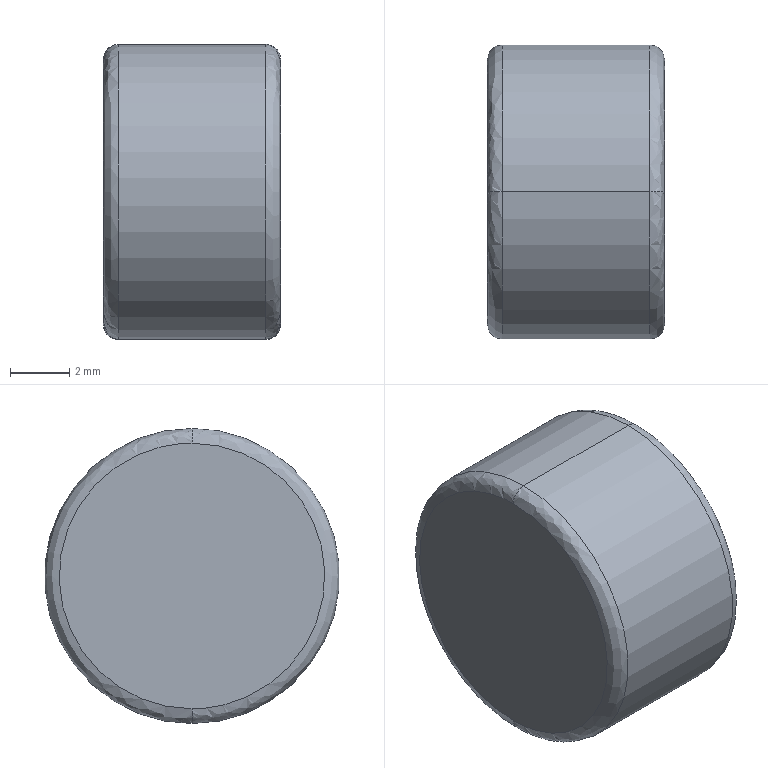Part | STEP file | Magnet dia 10 thickness 6 | 1 solid | 8 faces | box 6 x 10 x 10 mm | volume 467.969 mm3 | spline 4 | cylinder 2 | plane 2 | commonest cylinder face diameters 10 x2
STEP:
#1=CARTESIAN_POINT('',(0.,0.,0.));
#2=DIRECTION('',(0.,0.,1.));
#3=DIRECTION('',(1.,0.,0.));
#4=AXIS2_PLACEMENT_3D('',#1,#2,#3);
#5=CARTESIAN_POINT('',(5.5,-0.000000001,-5.));
#6=VERTEX_POINT('',#5);
#7=CARTESIAN_POINT('',(5.5,0.,5.));
#8=VERTEX_POINT('',#7);
#9=CARTESIAN_POINT('',(5.5,0.,0.));
#10=DIRECTION('',(1.,0.,0.));
#11=DIRECTION('',(0.,0.,1.));
#12=AXIS2_PLACEMENT_3D('',#9,#10,#11);
#13=CIRCLE('',#12,5.);
#14=CARTESIAN_POINT('',(5.5,0.,0.));
#15=DIRECTION('',(-1.,0.,0.));
#16=DIRECTION('',(0.,0.,1.));
#17=AXIS2_PLACEMENT_3D('',#14,#15,#16);
#18=CYLINDRICAL_SURFACE('',#17,5.);
#19=CARTESIAN_POINT('',(6.283,0.));
#20=DIRECTION('',(-1.,0.));
#21=VECTOR('',#20,1.);
#22=LINE('',#19,#21);
#23=(GEOMETRIC_REPRESENTATION_CONTEXT(2)PARAMETRIC_REPRESENTATION_CONTEXT()REPRESENTATION_CONTEXT('',''));
#24=DEFINITIONAL_REPRESENTATION('',(#22),#23);
#25=PCURVE('',#18,#24);
#26=CARTESIAN_POINT('',(5.998,0.,-4.45));
#27=CARTESIAN_POINT('',(5.998,8.9,-4.45));
#28=CARTESIAN_POINT('',(5.998,8.9,4.45));
#29=CARTESIAN_POINT('',(5.998,0.,4.45));
#30=CARTESIAN_POINT('',(6.032,0.,-4.79));
#31=CARTESIAN_POINT('',(6.032,9.58,-4.79));
#32=CARTESIAN_POINT('',(6.032,9.58,4.79));
#33=CARTESIAN_POINT('',(6.032,0.,4.79));
#34=CARTESIAN_POINT('',(5.79,0.,-5.032));
#35=CARTESIAN_POINT('',(5.79,10.063,-5.032));
#36=CARTESIAN_POINT('',(5.79,10.063,5.032));
#37=CARTESIAN_POINT('',(5.79,0.,5.032));
#38=CARTESIAN_POINT('',(5.45,0.,-4.998));
#39=CARTESIAN_POINT('',(5.45,9.995,-4.998));
#40=CARTESIAN_POINT('',(5.45,9.995,4.998));
#41=CARTESIAN_POINT('',(5.45,0.,4.998));
#42=(BOUNDED_SURFACE()B_SPLINE_SURFACE(3,3,((#26,#27,#28,#29),(#30,#31,#32,#33),(#34,#35,#36,#37),(#38,#39,#40,#41)),.UNSPECIFIED.,.F.,.F.,.F.)B_SPLINE_SURFACE_WITH_KNOTS((4,4),(4,4),(0.,1.),(0.,1.),.PIECEWISE_BEZIER_KNOTS.)GEOMETRIC_REPRESENTATION_ITEM()RATIONAL_B_SPLINE_SURFACE(((1.,0.3333,0.3333,1.),(0.7553,0.2518,0.2518,0.7553),(0.7553,0.2518,0.2518,0.7553),(1.,0.3333,0.3333,1.)))REPRESENTATION_ITEM('')SURFACE());
#43=CARTESIAN_POINT('',(0.9369,0.));
#44=CARTESIAN_POINT('',(0.9369,0.02375));
#45=CARTESIAN_POINT('',(0.9369,0.06805));
#46=CARTESIAN_POINT('',(0.9369,0.1267));
#47=CARTESIAN_POINT('',(0.9369,0.1794));
#48=CARTESIAN_POINT('',(0.9369,0.2276));
#49=CARTESIAN_POINT('',(0.9369,0.2721));
#50=CARTESIAN_POINT('',(0.9369,0.3139));
#51=CARTESIAN_POINT('',(0.9369,0.3535));
#52=CARTESIAN_POINT('',(0.9369,0.3914));
#53=CARTESIAN_POINT('',(0.9369,0.4282));
#54=CARTESIAN_POINT('',(0.9369,0.4643));
#55=CARTESIAN_POINT('',(0.9369,0.5));
#56=CARTESIAN_POINT('',(0.9369,0.5357));
#57=CARTESIAN_POINT('',(0.9369,0.5718));
#58=CARTESIAN_POINT('',(0.9369,0.6086));
#59=CARTESIAN_POINT('',(0.9369,0.6465));
#60=CARTESIAN_POINT('',(0.9369,0.6861));
#61=CARTESIAN_POINT('',(0.9369,0.7279));
#62=CARTESIAN_POINT('',(0.9369,0.7724));
#63=CARTESIAN_POINT('',(0.9369,0.8206));
#64=CARTESIAN_POINT('',(0.9369,0.8733));
#65=CARTESIAN_POINT('',(0.9369,0.9319));
#66=CARTESIAN_POINT('',(0.9369,0.9763));
#67=CARTESIAN_POINT('',(0.9369,1.));
#68=B_SPLINE_CURVE_WITH_KNOTS('',3,(#43,#44,#45,#46,#47,#48,#49,#50,#51,#52,#53,#54,#55,#56,#57,#58,#59,#60,#61,#62,#63,#64,#65,#66,#67),.UNSPECIFIED.,.F.,.F.,(4,1,1,1,1,1,1,1,1,1,1,1,1,1,1,1,1,1,1,1,1,1,4),(3.142,3.284,3.427,3.57,3.713,3.856,3.998,4.141,4.284,4.427,4.57,4.712,4.855,4.998,5.141,5.284,5.426,5.569,5.712,5.855,5.998,6.14,6.283),.QUASI_UNIFORM_KNOTS.);
#69=(GEOMETRIC_REPRESENTATION_CONTEXT(2)PARAMETRIC_REPRESENTATION_CONTEXT()REPRESENTATION_CONTEXT('',''));
#70=DEFINITIONAL_REPRESENTATION('',(#68),#69);
#71=PCURVE('',#42,#70);
#72=SURFACE_CURVE('',#13,(#25,#71),.PCURVE_S1.);
#73=EDGE_CURVE('',#6,#8,#72,.T.);
#74=ORIENTED_EDGE('',*,*,#73,.F.);
#75=CARTESIAN_POINT('',(0.5,0.,-5.));
#76=VERTEX_POINT('',#75);
#77=CARTESIAN_POINT('',(5.5,0.,-5.));
#78=DIRECTION('',(-1.,0.,0.));
#79=VECTOR('',#78,1.);
#80=LINE('',#77,#79);
#81=CARTESIAN_POINT('',(3.142,0.));
#82=DIRECTION('',(0.,1.));
#83=VECTOR('',#82,1.);
#84=LINE('',#81,#83);
#85=(GEOMETRIC_REPRESENTATION_CONTEXT(2)PARAMETRIC_REPRESENTATION_CONTEXT()REPRESENTATION_CONTEXT('',''));
#86=DEFINITIONAL_REPRESENTATION('',(#84),#85);
#87=PCURVE('',#18,#86);
#88=CARTESIAN_POINT('',(5.5,0.,0.));
#89=DIRECTION('',(-1.,0.,0.));
#90=DIRECTION('',(0.,0.,1.));
#91=AXIS2_PLACEMENT_3D('',#88,#89,#90);
#92=CYLINDRICAL_SURFACE('',#91,5.);
#93=CARTESIAN_POINT('',(3.142,0.));
#94=DIRECTION('',(0.,1.));
#95=VECTOR('',#94,1.);
#96=LINE('',#93,#95);
#97=(GEOMETRIC_REPRESENTATION_CONTEXT(2)PARAMETRIC_REPRESENTATION_CONTEXT()REPRESENTATION_CONTEXT('',''));
#98=DEFINITIONAL_REPRESENTATION('',(#96),#97);
#99=PCURVE('',#92,#98);
#100=SURFACE_CURVE('',#80,(#87,#99),.PCURVE_S1.);
#101=EDGE_CURVE('',#6,#76,#100,.T.);
#102=ORIENTED_EDGE('',*,*,#101,.T.);
#103=CARTESIAN_POINT('',(0.5,0.,5.));
#104=VERTEX_POINT('',#103);
#105=CARTESIAN_POINT('',(0.5,0.,0.));
#106=DIRECTION('',(-1.,0.,0.));
#107=DIRECTION('',(0.,-1.,0.));
#108=AXIS2_PLACEMENT_3D('',#105,#106,#107);
#109=CIRCLE('',#108,5.);
#110=CARTESIAN_POINT('',(-1.571,5.));
#111=DIRECTION('',(1.,0.));
#112=VECTOR('',#111,1.);
#113=LINE('',#110,#112);
#114=(GEOMETRIC_REPRESENTATION_CONTEXT(2)PARAMETRIC_REPRESENTATION_CONTEXT()REPRESENTATION_CONTEXT('',''));
#115=DEFINITIONAL_REPRESENTATION('',(#113),#114);
#116=PCURVE('',#18,#115);
#117=CARTESIAN_POINT('',(0.5499,0.,-4.998));
#118=CARTESIAN_POINT('',(0.5499,9.995,-4.998));
#119=CARTESIAN_POINT('',(0.5499,9.995,4.998));
#120=CARTESIAN_POINT('',(0.5499,0.,4.998));
#121=CARTESIAN_POINT('',(0.21,0.,-5.032));
#122=CARTESIAN_POINT('',(0.21,10.063,-5.032));
#123=CARTESIAN_POINT('',(0.21,10.063,5.032));
#124=CARTESIAN_POINT('',(0.21,0.,5.032));
#125=CARTESIAN_POINT('',(-0.03161,0.,-4.79));
#126=CARTESIAN_POINT('',(-0.03161,9.58,-4.79));
#127=CARTESIAN_POINT('',(-0.03161,9.58,4.79));
#128=CARTESIAN_POINT('',(-0.03161,0.,4.79));
#129=CARTESIAN_POINT('',(0.002498,0.,-4.45));
#130=CARTESIAN_POINT('',(0.002498,8.9,-4.45));
#131=CARTESIAN_POINT('',(0.002498,8.9,4.45));
#132=CARTESIAN_POINT('',(0.002498,0.,4.45));
#133=(BOUNDED_SURFACE()B_SPLINE_SURFACE(3,3,((#117,#118,#119,#120),(#121,#122,#123,#124),(#125,#126,#127,#128),(#129,#130,#131,#132)),.UNSPECIFIED.,.F.,.F.,.F.)B_SPLINE_SURFACE_WITH_KNOTS((4,4),(4,4),(0.,1.),(0.,1.),.PIECEWISE_BEZIER_KNOTS.)GEOMETRIC_REPRESENTATION_ITEM()RATIONAL_B_SPLINE_SURFACE(((1.,0.3333,0.3333,1.),(0.7553,0.2518,0.2518,0.7553),(0.7553,0.2518,0.2518,0.7553),(1.,0.3333,0.3333,1.)))REPRESENTATION_ITEM('')SURFACE());
#134=CARTESIAN_POINT('',(0.06314,1.));
#135=CARTESIAN_POINT('',(0.06314,0.9763));
#136=CARTESIAN_POINT('',(0.06314,0.9319));
#137=CARTESIAN_POINT('',(0.06314,0.8733));
#138=CARTESIAN_POINT('',(0.06314,0.8206));
#139=CARTESIAN_POINT('',(0.06314,0.7724));
#140=CARTESIAN_POINT('',(0.06314,0.7279));
#141=CARTESIAN_POINT('',(0.06314,0.6861));
#142=CARTESIAN_POINT('',(0.06314,0.6465));
#143=CARTESIAN_POINT('',(0.06314,0.6086));
#144=CARTESIAN_POINT('',(0.06314,0.5718));
#145=CARTESIAN_POINT('',(0.06314,0.5357));
#146=CARTESIAN_POINT('',(0.06314,0.5));
#147=CARTESIAN_POINT('',(0.06314,0.4643));
#148=CARTESIAN_POINT('',(0.06314,0.4282));
#149=CARTESIAN_POINT('',(0.06314,0.3914));
#150=CARTESIAN_POINT('',(0.06314,0.3535));
#151=CARTESIAN_POINT('',(0.06314,0.3139));
#152=CARTESIAN_POINT('',(0.06314,0.2721));
#153=CARTESIAN_POINT('',(0.06314,0.2276));
#154=CARTESIAN_POINT('',(0.06314,0.1794));
#155=CARTESIAN_POINT('',(0.06314,0.1267));
#156=CARTESIAN_POINT('',(0.06314,0.06805));
#157=CARTESIAN_POINT('',(0.06314,0.02375));
#158=CARTESIAN_POINT('',(0.06314,0.));
#159=B_SPLINE_CURVE_WITH_KNOTS('',3,(#134,#135,#136,#137,#138,#139,#140,#141,#142,#143,#144,#145,#146,#147,#148,#149,#150,#151,#152,#153,#154,#155,#156,#157,#158),.UNSPECIFIED.,.F.,.F.,(4,1,1,1,1,1,1,1,1,1,1,1,1,1,1,1,1,1,1,1,1,1,4),(1.571,1.714,1.856,1.999,2.142,2.285,2.428,2.57,2.713,2.856,2.999,3.142,3.284,3.427,3.57,3.713,3.856,3.998,4.141,4.284,4.427,4.57,4.712),.QUASI_UNIFORM_KNOTS.);
#160=(GEOMETRIC_REPRESENTATION_CONTEXT(2)PARAMETRIC_REPRESENTATION_CONTEXT()REPRESENTATION_CONTEXT('',''));
#161=DEFINITIONAL_REPRESENTATION('',(#159),#160);
#162=PCURVE('',#133,#161);
#163=SURFACE_CURVE('',#109,(#116,#162),.PCURVE_S1.);
#164=EDGE_CURVE('',#104,#76,#163,.T.);
#165=ORIENTED_EDGE('',*,*,#164,.F.);
#166=CARTESIAN_POINT('',(5.5,0.,5.));
#167=DIRECTION('',(-1.,0.,0.));
#168=VECTOR('',#167,1.);
#169=LINE('',#166,#168);
#170=CARTESIAN_POINT('',(0.,0.));
#171=DIRECTION('',(0.,1.));
#172=VECTOR('',#171,1.);
#173=LINE('',#170,#172);
#174=(GEOMETRIC_REPRESENTATION_CONTEXT(2)PARAMETRIC_REPRESENTATION_CONTEXT()REPRESENTATION_CONTEXT('',''));
#175=DEFINITIONAL_REPRESENTATION('',(#173),#174);
#176=PCURVE('',#18,#175);
#177=CARTESIAN_POINT('',(6.283,0.));
#178=DIRECTION('',(0.,1.));
#179=VECTOR('',#178,1.);
#180=LINE('',#177,#179);
#181=(GEOMETRIC_REPRESENTATION_CONTEXT(2)PARAMETRIC_REPRESENTATION_CONTEXT()REPRESENTATION_CONTEXT('',''));
#182=DEFINITIONAL_REPRESENTATION('',(#180),#181);
#183=PCURVE('',#92,#182);
#184=SURFACE_CURVE('',#169,(#176,#183),.PCURVE_S1.);
#185=EDGE_CURVE('',#8,#104,#184,.T.);
#186=ORIENTED_EDGE('',*,*,#185,.F.);
#187=EDGE_LOOP('',(#74,#102,#165,#186));
#188=FACE_BOUND('',#187,.T.);
#189=ADVANCED_FACE('',(#188),#18,.T.);
#190=ORIENTED_EDGE('',*,*,#164,.T.);
#191=CARTESIAN_POINT('',(0.,0.,-4.5));
#192=VERTEX_POINT('',#191);
#193=CARTESIAN_POINT('',(0.,0.,-4.5));
#194=CARTESIAN_POINT('',(0.,0.,-4.793));
#195=CARTESIAN_POINT('',(0.2071,0.,-5.));
#196=CARTESIAN_POINT('',(0.5,0.,-5.));
#197=(BOUNDED_CURVE()B_SPLINE_CURVE(3,(#193,#194,#195,#196),.UNSPECIFIED.,.F.,.F.)B_SPLINE_CURVE_WITH_KNOTS((4,4),(0.06314,0.9369),.PIECEWISE_BEZIER_KNOTS.)CURVE()GEOMETRIC_REPRESENTATION_ITEM()RATIONAL_B_SPLINE_CURVE((0.9566,0.7698,0.7698,0.9566))REPRESENTATION_ITEM(''));
#198=CARTESIAN_POINT('',(0.9369,0.));
#199=CARTESIAN_POINT('',(0.06314,0.));
#200=B_SPLINE_CURVE_WITH_KNOTS('',1,(#198,#199),.UNSPECIFIED.,.F.,.F.,(2,2),(0.06314,0.9369),.PIECEWISE_BEZIER_KNOTS.);
#201=(GEOMETRIC_REPRESENTATION_CONTEXT(2)PARAMETRIC_REPRESENTATION_CONTEXT()REPRESENTATION_CONTEXT('',''));
#202=DEFINITIONAL_REPRESENTATION('',(#200),#201);
#203=PCURVE('',#133,#202);
#204=CARTESIAN_POINT('',(0.5499,0.,4.998));
#205=CARTESIAN_POINT('',(0.5499,-9.995,4.998));
#206=CARTESIAN_POINT('',(0.5499,-9.995,-4.998));
#207=CARTESIAN_POINT('',(0.5499,0.,-4.998));
#208=CARTESIAN_POINT('',(0.21,0.,5.032));
#209=CARTESIAN_POINT('',(0.21,-10.063,5.032));
#210=CARTESIAN_POINT('',(0.21,-10.063,-5.032));
#211=CARTESIAN_POINT('',(0.21,0.,-5.032));
#212=CARTESIAN_POINT('',(-0.03161,0.,4.79));
#213=CARTESIAN_POINT('',(-0.03161,-9.58,4.79));
#214=CARTESIAN_POINT('',(-0.03161,-9.58,-4.79));
#215=CARTESIAN_POINT('',(-0.03161,0.,-4.79));
#216=CARTESIAN_POINT('',(0.002498,0.,4.45));
#217=CARTESIAN_POINT('',(0.002498,-8.9,4.45));
#218=CARTESIAN_POINT('',(0.002498,-8.9,-4.45));
#219=CARTESIAN_POINT('',(0.002498,0.,-4.45));
#220=(BOUNDED_SURFACE()B_SPLINE_SURFACE(3,3,((#204,#205,#206,#207),(#208,#209,#210,#211),(#212,#213,#214,#215),(#216,#217,#218,#219)),.UNSPECIFIED.,.F.,.F.,.F.)B_SPLINE_SURFACE_WITH_KNOTS((4,4),(4,4),(0.,1.),(0.,1.),.PIECEWISE_BEZIER_KNOTS.)GEOMETRIC_REPRESENTATION_ITEM()RATIONAL_B_SPLINE_SURFACE(((1.,0.3333,0.3333,1.),(0.7553,0.2518,0.2518,0.7553),(0.7553,0.2518,0.2518,0.7553),(1.,0.3333,0.3333,1.)))REPRESENTATION_ITEM('')SURFACE());
#221=CARTESIAN_POINT('',(0.9369,1.));
#222=CARTESIAN_POINT('',(0.06314,1.));
#223=B_SPLINE_CURVE_WITH_KNOTS('',1,(#221,#222),.UNSPECIFIED.,.F.,.F.,(2,2),(0.06314,0.9369),.PIECEWISE_BEZIER_KNOTS.);
#224=(GEOMETRIC_REPRESENTATION_CONTEXT(2)PARAMETRIC_REPRESENTATION_CONTEXT()REPRESENTATION_CONTEXT('',''));
#225=DEFINITIONAL_REPRESENTATION('',(#223),#224);
#226=PCURVE('',#220,#225);
#227=SURFACE_CURVE('',#197,(#203,#226),.PCURVE_S1.);
#228=EDGE_CURVE('',#192,#76,#227,.T.);
#229=ORIENTED_EDGE('',*,*,#228,.F.);
#230=CARTESIAN_POINT('',(0.,0.,4.5));
#231=VERTEX_POINT('',#230);
#232=CARTESIAN_POINT('',(0.,0.,-4.5));
#233=CARTESIAN_POINT('',(0.,9.,-4.5));
#234=CARTESIAN_POINT('',(0.,9.,4.5));
#235=CARTESIAN_POINT('',(0.,0.,4.5));
#236=(BOUNDED_CURVE()B_SPLINE_CURVE(3,(#232,#233,#234,#235),.UNSPECIFIED.,.F.,.F.)B_SPLINE_CURVE_WITH_KNOTS((4,4),(0.,1.),.PIECEWISE_BEZIER_KNOTS.)CURVE()GEOMETRIC_REPRESENTATION_ITEM()RATIONAL_B_SPLINE_CURVE((0.9566,0.3189,0.3189,0.9566))REPRESENTATION_ITEM(''));
#237=CARTESIAN_POINT('',(0.9369,0.));
#238=DIRECTION('',(0.,1.));
#239=VECTOR('',#238,1.);
#240=LINE('',#237,#239);
#241=(GEOMETRIC_REPRESENTATION_CONTEXT(2)PARAMETRIC_REPRESENTATION_CONTEXT()REPRESENTATION_CONTEXT('',''));
#242=DEFINITIONAL_REPRESENTATION('',(#240),#241);
#243=PCURVE('',#133,#242);
#244=CARTESIAN_POINT('',(0.,-4.554,4.554));
#245=DIRECTION('',(1.,0.,0.));
#246=DIRECTION('',(0.,0.,-1.));
#247=AXIS2_PLACEMENT_3D('',#244,#245,#246);
#248=PLANE('',#247);
#249=CARTESIAN_POINT('',(9.054,4.554));
#250=CARTESIAN_POINT('',(9.054,13.554));
#251=CARTESIAN_POINT('',(0.054,13.554));
#252=CARTESIAN_POINT('',(0.054,4.554));
#253=(BOUNDED_CURVE()B_SPLINE_CURVE(3,(#249,#250,#251,#252),.UNSPECIFIED.,.F.,.F.)B_SPLINE_CURVE_WITH_KNOTS((4,4),(0.,1.),.PIECEWISE_BEZIER_KNOTS.)CURVE()GEOMETRIC_REPRESENTATION_ITEM()RATIONAL_B_SPLINE_CURVE((0.9566,0.3189,0.3189,0.9566))REPRESENTATION_ITEM(''));
#254=(GEOMETRIC_REPRESENTATION_CONTEXT(2)PARAMETRIC_REPRESENTATION_CONTEXT()REPRESENTATION_CONTEXT('',''));
#255=DEFINITIONAL_REPRESENTATION('',(#253),#254);
#256=PCURVE('',#248,#255);
#257=SURFACE_CURVE('',#236,(#243,#256),.PCURVE_S1.);
#258=EDGE_CURVE('',#192,#231,#257,.T.);
#259=ORIENTED_EDGE('',*,*,#258,.T.);
#260=CARTESIAN_POINT('',(0.5,0.,5.));
#261=CARTESIAN_POINT('',(0.2071,0.,5.));
#262=CARTESIAN_POINT('',(0.,0.,4.793));
#263=CARTESIAN_POINT('',(0.,0.,4.5));
#264=(BOUNDED_CURVE()B_SPLINE_CURVE(3,(#260,#261,#262,#263),.UNSPECIFIED.,.F.,.F.)B_SPLINE_CURVE_WITH_KNOTS((4,4),(0.06314,0.9369),.PIECEWISE_BEZIER_KNOTS.)CURVE()GEOMETRIC_REPRESENTATION_ITEM()RATIONAL_B_SPLINE_CURVE((0.9566,0.7698,0.7698,0.9566))REPRESENTATION_ITEM(''));
#265=CARTESIAN_POINT('',(0.06314,1.));
#266=CARTESIAN_POINT('',(0.9369,1.));
#267=B_SPLINE_CURVE_WITH_KNOTS('',1,(#265,#266),.UNSPECIFIED.,.F.,.F.,(2,2),(0.06314,0.9369),.PIECEWISE_BEZIER_KNOTS.);
#268=(GEOMETRIC_REPRESENTATION_CONTEXT(2)PARAMETRIC_REPRESENTATION_CONTEXT()REPRESENTATION_CONTEXT('',''));
#269=DEFINITIONAL_REPRESENTATION('',(#267),#268);
#270=PCURVE('',#133,#269);
#271=CARTESIAN_POINT('',(0.06314,0.));
#272=CARTESIAN_POINT('',(0.9369,0.));
#273=B_SPLINE_CURVE_WITH_KNOTS('',1,(#271,#272),.UNSPECIFIED.,.F.,.F.,(2,2),(0.06314,0.9369),.PIECEWISE_BEZIER_KNOTS.);
#274=(GEOMETRIC_REPRESENTATION_CONTEXT(2)PARAMETRIC_REPRESENTATION_CONTEXT()REPRESENTATION_CONTEXT('',''));
#275=DEFINITIONAL_REPRESENTATION('',(#273),#274);
#276=PCURVE('',#220,#275);
#277=SURFACE_CURVE('',#264,(#270,#276),.PCURVE_S1.);
#278=EDGE_CURVE('',#104,#231,#277,.T.);
#279=ORIENTED_EDGE('',*,*,#278,.F.);
#280=EDGE_LOOP('',(#190,#229,#259,#279));
#281=FACE_BOUND('',#280,.T.);
#282=ADVANCED_FACE('',(#281),#133,.T.);
#283=ORIENTED_EDGE('',*,*,#101,.F.);
#284=CARTESIAN_POINT('',(5.5,0.,0.));
#285=DIRECTION('',(1.,0.,0.));
#286=DIRECTION('',(0.,0.,1.));
#287=AXIS2_PLACEMENT_3D('',#284,#285,#286);
#288=CIRCLE('',#287,5.);
#289=CARTESIAN_POINT('',(6.283,0.));
#290=DIRECTION('',(-1.,0.));
#291=VECTOR('',#290,1.);
#292=LINE('',#289,#291);
#293=(GEOMETRIC_REPRESENTATION_CONTEXT(2)PARAMETRIC_REPRESENTATION_CONTEXT()REPRESENTATION_CONTEXT('',''));
#294=DEFINITIONAL_REPRESENTATION('',(#292),#293);
#295=PCURVE('',#92,#294);
#296=CARTESIAN_POINT('',(5.998,0.,4.45));
#297=CARTESIAN_POINT('',(5.998,-8.9,4.45));
#298=CARTESIAN_POINT('',(5.998,-8.9,-4.45));
#299=CARTESIAN_POINT('',(5.998,0.,-4.45));
#300=CARTESIAN_POINT('',(6.032,0.,4.79));
#301=CARTESIAN_POINT('',(6.032,-9.58,4.79));
#302=CARTESIAN_POINT('',(6.032,-9.58,-4.79));
#303=CARTESIAN_POINT('',(6.032,0.,-4.79));
#304=CARTESIAN_POINT('',(5.79,0.,5.032));
#305=CARTESIAN_POINT('',(5.79,-10.063,5.032));
#306=CARTESIAN_POINT('',(5.79,-10.063,-5.032));
#307=CARTESIAN_POINT('',(5.79,0.,-5.032));
#308=CARTESIAN_POINT('',(5.45,0.,4.998));
#309=CARTESIAN_POINT('',(5.45,-9.995,4.998));
#310=CARTESIAN_POINT('',(5.45,-9.995,-4.998));
#311=CARTESIAN_POINT('',(5.45,0.,-4.998));
#312=(BOUNDED_SURFACE()B_SPLINE_SURFACE(3,3,((#296,#297,#298,#299),(#300,#301,#302,#303),(#304,#305,#306,#307),(#308,#309,#310,#311)),.UNSPECIFIED.,.F.,.F.,.F.)B_SPLINE_SURFACE_WITH_KNOTS((4,4),(4,4),(0.,1.),(0.,1.),.PIECEWISE_BEZIER_KNOTS.)GEOMETRIC_REPRESENTATION_ITEM()RATIONAL_B_SPLINE_SURFACE(((1.,0.3333,0.3333,1.),(0.7553,0.2518,0.2518,0.7553),(0.7553,0.2518,0.2518,0.7553),(1.,0.3333,0.3333,1.)))REPRESENTATION_ITEM('')SURFACE());
#313=CARTESIAN_POINT('',(0.9369,0.));
#314=CARTESIAN_POINT('',(0.9369,0.02375));
#315=CARTESIAN_POINT('',(0.9369,0.06805));
#316=CARTESIAN_POINT('',(0.9369,0.1267));
#317=CARTESIAN_POINT('',(0.9369,0.1794));
#318=CARTESIAN_POINT('',(0.9369,0.2276));
#319=CARTESIAN_POINT('',(0.9369,0.2721));
#320=CARTESIAN_POINT('',(0.9369,0.3139));
#321=CARTESIAN_POINT('',(0.9369,0.3535));
#322=CARTESIAN_POINT('',(0.9369,0.3914));
#323=CARTESIAN_POINT('',(0.9369,0.4282));
#324=CARTESIAN_POINT('',(0.9369,0.4643));
#325=CARTESIAN_POINT('',(0.9369,0.5));
#326=CARTESIAN_POINT('',(0.9369,0.5357));
#327=CARTESIAN_POINT('',(0.9369,0.5718));
#328=CARTESIAN_POINT('',(0.9369,0.6086));
#329=CARTESIAN_POINT('',(0.9369,0.6465));
#330=CARTESIAN_POINT('',(0.9369,0.6861));
#331=CARTESIAN_POINT('',(0.9369,0.7279));
#332=CARTESIAN_POINT('',(0.9369,0.7724));
#333=CARTESIAN_POINT('',(0.9369,0.8206));
#334=CARTESIAN_POINT('',(0.9369,0.8733));
#335=CARTESIAN_POINT('',(0.9369,0.9319));
#336=CARTESIAN_POINT('',(0.9369,0.9763));
#337=CARTESIAN_POINT('',(0.9369,1.));
#338=B_SPLINE_CURVE_WITH_KNOTS('',3,(#313,#314,#315,#316,#317,#318,#319,#320,#321,#322,#323,#324,#325,#326,#327,#328,#329,#330,#331,#332,#333,#334,#335,#336,#337),.UNSPECIFIED.,.F.,.F.,(4,1,1,1,1,1,1,1,1,1,1,1,1,1,1,1,1,1,1,1,1,1,4),(0.,0.1428,0.2856,0.4284,0.5712,0.714,0.8568,0.9996,1.142,1.285,1.428,1.571,1.714,1.856,1.999,2.142,2.285,2.428,2.57,2.713,2.856,2.999,3.142),.QUASI_UNIFORM_KNOTS.);
#339=(GEOMETRIC_REPRESENTATION_CONTEXT(2)PARAMETRIC_REPRESENTATION_CONTEXT()REPRESENTATION_CONTEXT('',''));
#340=DEFINITIONAL_REPRESENTATION('',(#338),#339);
#341=PCURVE('',#312,#340);
#342=SURFACE_CURVE('',#288,(#295,#341),.PCURVE_S1.);
#343=EDGE_CURVE('',#8,#6,#342,.T.);
#344=ORIENTED_EDGE('',*,*,#343,.F.);
#345=ORIENTED_EDGE('',*,*,#185,.T.);
#346=CARTESIAN_POINT('',(0.5,0.,0.));
#347=DIRECTION('',(-1.,0.,0.));
#348=DIRECTION('',(0.,0.,1.));
#349=AXIS2_PLACEMENT_3D('',#346,#347,#348);
#350=CIRCLE('',#349,5.);
#351=CARTESIAN_POINT('',(0.,5.));
#352=DIRECTION('',(1.,0.));
#353=VECTOR('',#352,1.);
#354=LINE('',#351,#353);
#355=(GEOMETRIC_REPRESENTATION_CONTEXT(2)PARAMETRIC_REPRESENTATION_CONTEXT()REPRESENTATION_CONTEXT('',''));
#356=DEFINITIONAL_REPRESENTATION('',(#354),#355);
#357=PCURVE('',#92,#356);
#358=CARTESIAN_POINT('',(0.06314,1.));
#359=CARTESIAN_POINT('',(0.06314,0.9763));
#360=CARTESIAN_POINT('',(0.06314,0.9319));
#361=CARTESIAN_POINT('',(0.06314,0.8733));
#362=CARTESIAN_POINT('',(0.06314,0.8206));
#363=CARTESIAN_POINT('',(0.06314,0.7724));
#364=CARTESIAN_POINT('',(0.06314,0.7279));
#365=CARTESIAN_POINT('',(0.06314,0.6861));
#366=CARTESIAN_POINT('',(0.06314,0.6465));
#367=CARTESIAN_POINT('',(0.06314,0.6086));
#368=CARTESIAN_POINT('',(0.06314,0.5718));
#369=CARTESIAN_POINT('',(0.06314,0.5357));
#370=CARTESIAN_POINT('',(0.06314,0.5));
#371=CARTESIAN_POINT('',(0.06314,0.4643));
#372=CARTESIAN_POINT('',(0.06314,0.4282));
#373=CARTESIAN_POINT('',(0.06314,0.3914));
#374=CARTESIAN_POINT('',(0.06314,0.3535));
#375=CARTESIAN_POINT('',(0.06314,0.3139));
#376=CARTESIAN_POINT('',(0.06314,0.2721));
#377=CARTESIAN_POINT('',(0.06314,0.2276));
#378=CARTESIAN_POINT('',(0.06314,0.1794));
#379=CARTESIAN_POINT('',(0.06314,0.1267));
#380=CARTESIAN_POINT('',(0.06314,0.06805));
#381=CARTESIAN_POINT('',(0.06314,0.02375));
#382=CARTESIAN_POINT('',(0.06314,0.));
#383=B_SPLINE_CURVE_WITH_KNOTS('',3,(#358,#359,#360,#361,#362,#363,#364,#365,#366,#367,#368,#369,#370,#371,#372,#373,#374,#375,#376,#377,#378,#379,#380,#381,#382),.UNSPECIFIED.,.F.,.F.,(4,1,1,1,1,1,1,1,1,1,1,1,1,1,1,1,1,1,1,1,1,1,4),(3.142,3.284,3.427,3.57,3.713,3.856,3.998,4.141,4.284,4.427,4.57,4.712,4.855,4.998,5.141,5.284,5.426,5.569,5.712,5.855,5.998,6.14,6.283),.QUASI_UNIFORM_KNOTS.);
#384=(GEOMETRIC_REPRESENTATION_CONTEXT(2)PARAMETRIC_REPRESENTATION_CONTEXT()REPRESENTATION_CONTEXT('',''));
#385=DEFINITIONAL_REPRESENTATION('',(#383),#384);
#386=PCURVE('',#220,#385);
#387=SURFACE_CURVE('',#350,(#357,#386),.PCURVE_S1.);
#388=EDGE_CURVE('',#76,#104,#387,.T.);
#389=ORIENTED_EDGE('',*,*,#388,.F.);
#390=EDGE_LOOP('',(#283,#344,#345,#389));
#391=FACE_BOUND('',#390,.T.);
#392=ADVANCED_FACE('',(#391),#92,.T.);
#393=ORIENTED_EDGE('',*,*,#258,.F.);
#394=CARTESIAN_POINT('',(0.,0.,4.5));
#395=CARTESIAN_POINT('',(0.,-9.,4.5));
#396=CARTESIAN_POINT('',(0.,-9.,-4.5));
#397=CARTESIAN_POINT('',(0.,0.,-4.5));
#398=(BOUNDED_CURVE()B_SPLINE_CURVE(3,(#394,#395,#396,#397),.UNSPECIFIED.,.F.,.F.)B_SPLINE_CURVE_WITH_KNOTS((4,4),(0.,1.),.PIECEWISE_BEZIER_KNOTS.)CURVE()GEOMETRIC_REPRESENTATION_ITEM()RATIONAL_B_SPLINE_CURVE((0.9566,0.3189,0.3189,0.9566))REPRESENTATION_ITEM(''));
#399=CARTESIAN_POINT('',(0.054,4.554));
#400=CARTESIAN_POINT('',(0.054,-4.446));
#401=CARTESIAN_POINT('',(9.054,-4.446));
#402=CARTESIAN_POINT('',(9.054,4.554));
#403=(BOUNDED_CURVE()B_SPLINE_CURVE(3,(#399,#400,#401,#402),.UNSPECIFIED.,.F.,.F.)B_SPLINE_CURVE_WITH_KNOTS((4,4),(0.,1.),.PIECEWISE_BEZIER_KNOTS.)CURVE()GEOMETRIC_REPRESENTATION_ITEM()RATIONAL_B_SPLINE_CURVE((0.9566,0.3189,0.3189,0.9566))REPRESENTATION_ITEM(''));
#404=(GEOMETRIC_REPRESENTATION_CONTEXT(2)PARAMETRIC_REPRESENTATION_CONTEXT()REPRESENTATION_CONTEXT('',''));
#405=DEFINITIONAL_REPRESENTATION('',(#403),#404);
#406=PCURVE('',#248,#405);
#407=CARTESIAN_POINT('',(0.9369,0.));
#408=DIRECTION('',(0.,1.));
#409=VECTOR('',#408,1.);
#410=LINE('',#407,#409);
#411=(GEOMETRIC_REPRESENTATION_CONTEXT(2)PARAMETRIC_REPRESENTATION_CONTEXT()REPRESENTATION_CONTEXT('',''));
#412=DEFINITIONAL_REPRESENTATION('',(#410),#411);
#413=PCURVE('',#220,#412);
#414=SURFACE_CURVE('',#398,(#406,#413),.PCURVE_S1.);
#415=EDGE_CURVE('',#231,#192,#414,.T.);
#416=ORIENTED_EDGE('',*,*,#415,.F.);
#417=EDGE_LOOP('',(#393,#416));
#418=FACE_BOUND('',#417,.T.);
#419=ADVANCED_FACE('',(#418),#248,.F.);
#420=CARTESIAN_POINT('',(6.,0.,4.5));
#421=VERTEX_POINT('',#420);
#422=CARTESIAN_POINT('',(6.,0.,-4.5));
#423=VERTEX_POINT('',#422);
#424=CARTESIAN_POINT('',(6.,0.,4.5));
#425=CARTESIAN_POINT('',(6.,9.,4.5));
#426=CARTESIAN_POINT('',(6.,9.,-4.5));
#427=CARTESIAN_POINT('',(6.,0.,-4.5));
#428=(BOUNDED_CURVE()B_SPLINE_CURVE(3,(#424,#425,#426,#427),.UNSPECIFIED.,.F.,.F.)B_SPLINE_CURVE_WITH_KNOTS((4,4),(0.,1.),.PIECEWISE_BEZIER_KNOTS.)CURVE()GEOMETRIC_REPRESENTATION_ITEM()RATIONAL_B_SPLINE_CURVE((0.9566,0.3189,0.3189,0.9566))REPRESENTATION_ITEM(''));
#429=CARTESIAN_POINT('',(0.06314,1.));
#430=DIRECTION('',(0.,-1.));
#431=VECTOR('',#430,1.);
#432=LINE('',#429,#431);
#433=(GEOMETRIC_REPRESENTATION_CONTEXT(2)PARAMETRIC_REPRESENTATION_CONTEXT()REPRESENTATION_CONTEXT('',''));
#434=DEFINITIONAL_REPRESENTATION('',(#432),#433);
#435=PCURVE('',#42,#434);
#436=CARTESIAN_POINT('',(6.,-4.554,4.554));
#437=DIRECTION('',(1.,0.,0.));
#438=DIRECTION('',(0.,0.,-1.));
#439=AXIS2_PLACEMENT_3D('',#436,#437,#438);
#440=PLANE('',#439);
#441=CARTESIAN_POINT('',(0.054,4.554));
#442=CARTESIAN_POINT('',(0.054,13.554));
#443=CARTESIAN_POINT('',(9.054,13.554));
#444=CARTESIAN_POINT('',(9.054,4.554));
#445=(BOUNDED_CURVE()B_SPLINE_CURVE(3,(#441,#442,#443,#444),.UNSPECIFIED.,.F.,.F.)B_SPLINE_CURVE_WITH_KNOTS((4,4),(0.,1.),.PIECEWISE_BEZIER_KNOTS.)CURVE()GEOMETRIC_REPRESENTATION_ITEM()RATIONAL_B_SPLINE_CURVE((0.9566,0.3189,0.3189,0.9566))REPRESENTATION_ITEM(''));
#446=(GEOMETRIC_REPRESENTATION_CONTEXT(2)PARAMETRIC_REPRESENTATION_CONTEXT()REPRESENTATION_CONTEXT('',''));
#447=DEFINITIONAL_REPRESENTATION('',(#445),#446);
#448=PCURVE('',#440,#447);
#449=SURFACE_CURVE('',#428,(#435,#448),.PCURVE_S1.);
#450=EDGE_CURVE('',#421,#423,#449,.T.);
#451=ORIENTED_EDGE('',*,*,#450,.T.);
#452=CARTESIAN_POINT('',(5.5,-0.000000001,-5.));
#453=CARTESIAN_POINT('',(5.793,0.,-5.));
#454=CARTESIAN_POINT('',(6.,0.,-4.793));
#455=CARTESIAN_POINT('',(6.,0.,-4.5));
#456=(BOUNDED_CURVE()B_SPLINE_CURVE(3,(#452,#453,#454,#455),.UNSPECIFIED.,.F.,.F.)B_SPLINE_CURVE_WITH_KNOTS((4,4),(0.06314,0.9369),.PIECEWISE_BEZIER_KNOTS.)CURVE()GEOMETRIC_REPRESENTATION_ITEM()RATIONAL_B_SPLINE_CURVE((0.9566,0.7698,0.7698,0.9566))REPRESENTATION_ITEM(''));
#457=CARTESIAN_POINT('',(0.9369,0.));
#458=CARTESIAN_POINT('',(0.06314,0.));
#459=B_SPLINE_CURVE_WITH_KNOTS('',1,(#457,#458),.UNSPECIFIED.,.F.,.F.,(2,2),(0.06314,0.9369),.PIECEWISE_BEZIER_KNOTS.);
#460=(GEOMETRIC_REPRESENTATION_CONTEXT(2)PARAMETRIC_REPRESENTATION_CONTEXT()REPRESENTATION_CONTEXT('',''));
#461=DEFINITIONAL_REPRESENTATION('',(#459),#460);
#462=PCURVE('',#42,#461);
#463=CARTESIAN_POINT('',(0.9369,1.));
#464=CARTESIAN_POINT('',(0.06314,1.));
#465=B_SPLINE_CURVE_WITH_KNOTS('',1,(#463,#464),.UNSPECIFIED.,.F.,.F.,(2,2),(0.06314,0.9369),.PIECEWISE_BEZIER_KNOTS.);
#466=(GEOMETRIC_REPRESENTATION_CONTEXT(2)PARAMETRIC_REPRESENTATION_CONTEXT()REPRESENTATION_CONTEXT('',''));
#467=DEFINITIONAL_REPRESENTATION('',(#465),#466);
#468=PCURVE('',#312,#467);
#469=SURFACE_CURVE('',#456,(#462,#468),.PCURVE_S1.);
#470=EDGE_CURVE('',#6,#423,#469,.T.);
#471=ORIENTED_EDGE('',*,*,#470,.F.);
#472=ORIENTED_EDGE('',*,*,#73,.T.);
#473=CARTESIAN_POINT('',(6.,0.,4.5));
#474=CARTESIAN_POINT('',(6.,0.,4.793));
#475=CARTESIAN_POINT('',(5.793,0.,5.));
#476=CARTESIAN_POINT('',(5.5,0.,5.));
#477=(BOUNDED_CURVE()B_SPLINE_CURVE(3,(#473,#474,#475,#476),.UNSPECIFIED.,.F.,.F.)B_SPLINE_CURVE_WITH_KNOTS((4,4),(0.06314,0.9369),.PIECEWISE_BEZIER_KNOTS.)CURVE()GEOMETRIC_REPRESENTATION_ITEM()RATIONAL_B_SPLINE_CURVE((0.9566,0.7698,0.7698,0.9566))REPRESENTATION_ITEM(''));
#478=CARTESIAN_POINT('',(0.06314,1.));
#479=CARTESIAN_POINT('',(0.9369,1.));
#480=B_SPLINE_CURVE_WITH_KNOTS('',1,(#478,#479),.UNSPECIFIED.,.F.,.F.,(2,2),(0.06314,0.9369),.PIECEWISE_BEZIER_KNOTS.);
#481=(GEOMETRIC_REPRESENTATION_CONTEXT(2)PARAMETRIC_REPRESENTATION_CONTEXT()REPRESENTATION_CONTEXT('',''));
#482=DEFINITIONAL_REPRESENTATION('',(#480),#481);
#483=PCURVE('',#42,#482);
#484=CARTESIAN_POINT('',(0.06314,0.));
#485=CARTESIAN_POINT('',(0.9369,0.));
#486=B_SPLINE_CURVE_WITH_KNOTS('',1,(#484,#485),.UNSPECIFIED.,.F.,.F.,(2,2),(0.06314,0.9369),.PIECEWISE_BEZIER_KNOTS.);
#487=(GEOMETRIC_REPRESENTATION_CONTEXT(2)PARAMETRIC_REPRESENTATION_CONTEXT()REPRESENTATION_CONTEXT('',''));
#488=DEFINITIONAL_REPRESENTATION('',(#486),#487);
#489=PCURVE('',#312,#488);
#490=SURFACE_CURVE('',#477,(#483,#489),.PCURVE_S1.);
#491=EDGE_CURVE('',#421,#8,#490,.T.);
#492=ORIENTED_EDGE('',*,*,#491,.F.);
#493=EDGE_LOOP('',(#451,#471,#472,#492));
#494=FACE_BOUND('',#493,.T.);
#495=ADVANCED_FACE('',(#494),#42,.T.);
#496=ORIENTED_EDGE('',*,*,#228,.T.);
#497=ORIENTED_EDGE('',*,*,#388,.T.);
#498=ORIENTED_EDGE('',*,*,#278,.T.);
#499=ORIENTED_EDGE('',*,*,#415,.T.);
#500=EDGE_LOOP('',(#496,#497,#498,#499));
#501=FACE_BOUND('',#500,.T.);
#502=ADVANCED_FACE('',(#501),#220,.T.);
#503=ORIENTED_EDGE('',*,*,#450,.F.);
#504=CARTESIAN_POINT('',(6.,0.,4.5));
#505=CARTESIAN_POINT('',(6.,-0.09991,4.5));
#506=CARTESIAN_POINT('',(6.,-0.2495,4.495));
#507=CARTESIAN_POINT('',(6.,-0.4236,4.481));
#508=CARTESIAN_POINT('',(6.,-0.5105,4.471));
#509=CARTESIAN_POINT('',(6.,-0.5477,4.467));
#510=CARTESIAN_POINT('',(6.,-0.5725,4.463));
#511=CARTESIAN_POINT('',(6.,-0.5833,4.462));
#512=CARTESIAN_POINT('',(6.,-0.7094,4.445));
#513=CARTESIAN_POINT('',(6.,-0.8762,4.416));
#514=CARTESIAN_POINT('',(6.,-1.069,4.372));
#515=CARTESIAN_POINT('',(6.,-1.165,4.347));
#516=CARTESIAN_POINT('',(6.,-1.206,4.336));
#517=CARTESIAN_POINT('',(6.,-1.233,4.328));
#518=CARTESIAN_POINT('',(6.,-1.245,4.324));
#519=CARTESIAN_POINT('',(6.,-1.382,4.284));
#520=CARTESIAN_POINT('',(6.,-1.563,4.223));
#521=CARTESIAN_POINT('',(6.,-1.769,4.139));
#522=CARTESIAN_POINT('',(6.,-1.871,4.093));
#523=CARTESIAN_POINT('',(6.,-1.914,4.073));
#524=CARTESIAN_POINT('',(6.,-1.943,4.059));
#525=CARTESIAN_POINT('',(6.,-1.956,4.053));
#526=CARTESIAN_POINT('',(6.,-2.1,3.982));
#527=CARTESIAN_POINT('',(6.,-2.287,3.88));
#528=CARTESIAN_POINT('',(6.,-2.497,3.745));
#529=CARTESIAN_POINT('',(6.,-2.599,3.674));
#530=CARTESIAN_POINT('',(6.,-2.643,3.642));
#531=CARTESIAN_POINT('',(6.,-2.671,3.621));
#532=CARTESIAN_POINT('',(6.,-2.684,3.612));
#533=CARTESIAN_POINT('',(6.,-2.826,3.505));
#534=CARTESIAN_POINT('',(6.,-3.007,3.354));
#535=CARTESIAN_POINT('',(6.,-3.204,3.162));
#536=CARTESIAN_POINT('',(6.,-3.298,3.062));
#537=CARTESIAN_POINT('',(6.,-3.338,3.018));
#538=CARTESIAN_POINT('',(6.,-3.364,2.989));
#539=CARTESIAN_POINT('',(6.,-3.376,2.975));
#540=CARTESIAN_POINT('',(6.,-3.503,2.83));
#541=CARTESIAN_POINT('',(6.,-3.66,2.628));
#542=CARTESIAN_POINT('',(6.,-3.822,2.378));
#543=CARTESIAN_POINT('',(6.,-3.898,2.249));
#544=CARTESIAN_POINT('',(6.,-3.93,2.193));
#545=CARTESIAN_POINT('',(6.,-3.95,2.155));
#546=CARTESIAN_POINT('',(6.,-3.96,2.138));
#547=CARTESIAN_POINT('',(6.,-4.056,1.957));
#548=CARTESIAN_POINT('',(6.,-4.169,1.711));
#549=CARTESIAN_POINT('',(6.,-4.274,1.413));
#550=CARTESIAN_POINT('',(6.,-4.314,1.283));
#551=CARTESIAN_POINT('',(6.,-4.338,1.196));
#552=CARTESIAN_POINT('',(6.,-4.35,1.153));
#553=CARTESIAN_POINT('',(6.,-4.454,0.7446));
#554=CARTESIAN_POINT('',(6.,-4.5,0.3746));
#555=CARTESIAN_POINT('',(6.,-4.5,-0.1873));
#556=CARTESIAN_POINT('',(6.,-4.483,-0.4663));
#557=CARTESIAN_POINT('',(6.,-4.432,-0.7882));
#558=CARTESIAN_POINT('',(6.,-4.404,-0.9254));
#559=CARTESIAN_POINT('',(6.,-4.384,-1.017));
#560=CARTESIAN_POINT('',(6.,-4.373,-1.064));
#561=CARTESIAN_POINT('',(6.,-4.317,-1.284));
#562=CARTESIAN_POINT('',(6.,-4.234,-1.542));
#563=CARTESIAN_POINT('',(6.,-4.111,-1.833));
#564=CARTESIAN_POINT('',(6.,-4.043,-1.976));
#565=CARTESIAN_POINT('',(6.,-4.013,-2.037));
#566=CARTESIAN_POINT('',(6.,-3.992,-2.077));
#567=CARTESIAN_POINT('',(6.,-3.981,-2.099));
#568=CARTESIAN_POINT('',(6.,-3.89,-2.269));
#569=CARTESIAN_POINT('',(6.,-3.757,-2.487));
#570=CARTESIAN_POINT('',(6.,-3.581,-2.728));
#571=CARTESIAN_POINT('',(6.,-3.487,-2.845));
#572=CARTESIAN_POINT('',(6.,-3.446,-2.894));
#573=CARTESIAN_POINT('',(6.,-3.418,-2.926));
#574=CARTESIAN_POINT('',(6.,-3.403,-2.944));
#575=CARTESIAN_POINT('',(6.,-3.287,-3.078));
#576=CARTESIAN_POINT('',(6.,-3.123,-3.247));
#577=CARTESIAN_POINT('',(6.,-2.916,-3.429));
#578=CARTESIAN_POINT('',(6.,-2.809,-3.516));
#579=CARTESIAN_POINT('',(6.,-2.763,-3.552));
#580=CARTESIAN_POINT('',(6.,-2.732,-3.576));
#581=CARTESIAN_POINT('',(6.,-2.714,-3.589));
#582=CARTESIAN_POINT('',(6.,-2.586,-3.686));
#583=CARTESIAN_POINT('',(6.,-2.409,-3.805));
#584=CARTESIAN_POINT('',(6.,-2.194,-3.93));
#585=CARTESIAN_POINT('',(6.,-2.084,-3.989));
#586=CARTESIAN_POINT('',(6.,-2.036,-4.013));
#587=CARTESIAN_POINT('',(6.,-2.004,-4.029));
#588=CARTESIAN_POINT('',(6.,-1.986,-4.038));
#589=CARTESIAN_POINT('',(6.,-1.857,-4.101));
#590=CARTESIAN_POINT('',(6.,-1.682,-4.177));
#591=CARTESIAN_POINT('',(6.,-1.473,-4.253));
#592=CARTESIAN_POINT('',(6.,-1.367,-4.288));
#593=CARTESIAN_POINT('',(6.,-1.321,-4.302));
#594=CARTESIAN_POINT('',(6.,-1.291,-4.311));
#595=CARTESIAN_POINT('',(6.,-1.274,-4.316));
#596=CARTESIAN_POINT('',(6.,-1.151,-4.352));
#597=CARTESIAN_POINT('',(6.,-0.9873,-4.393));
#598=CARTESIAN_POINT('',(6.,-0.7932,-4.43));
#599=CARTESIAN_POINT('',(6.,-0.6955,-4.446));
#600=CARTESIAN_POINT('',(6.,-0.6535,-4.452));
#601=CARTESIAN_POINT('',(6.,-0.6254,-4.456));
#602=CARTESIAN_POINT('',(6.,-0.6097,-4.459));
#603=CARTESIAN_POINT('',(6.,-0.3993,-4.487));
#604=CARTESIAN_POINT('',(6.,-0.2002,-4.5));
#605=CARTESIAN_POINT('',(6.,0.,-4.5));
#606=B_SPLINE_CURVE_WITH_KNOTS('',3,(#504,#505,#506,#507,#508,#509,#510,#511,#512,#513,#514,#515,#516,#517,#518,#519,#520,#521,#522,#523,#524,#525,#526,#527,#528,#529,#530,#531,#532,#533,#534,#535,#536,#537,#538,#539,#540,#541,#542,#543,#544,#545,#546,#547,#548,#549,#550,#551,#552,#553,#554,#555,#556,#557,#558,#559,#560,#561,#562,#563,#564,#565,#566,#567,#568,#569,#570,#571,#572,#573,#574,#575,#576,#577,#578,#579,#580,#581,#582,#583,#584,#585,#586,#587,#588,#589,#590,#591,#592,#593,#594,#595,#596,#597,#598,#599,#600,#601,#602,#603,#604,#605),.UNSPECIFIED.,.F.,.F.,(4,1,1,1,2,2,1,1,1,2,2,1,1,1,2,2,1,1,1,2,2,1,1,1,2,2,1,1,1,2,2,1,1,2,2,2,1,1,2,2,1,1,1,2,2,1,1,1,2,2,1,1,1,2,2,1,1,1,2,2,1,1,1,2,2,1,1,1,2,2,4),(0.,0.03125,0.04688,0.05469,0.05859,0.0625,0.09375,0.1094,0.1172,0.1211,0.125,0.1562,0.1719,0.1797,0.1836,0.1875,0.2188,0.2344,0.2422,0.2461,0.25,0.2812,0.2969,0.3047,0.3086,0.3125,0.3438,0.3594,0.3672,0.3711,0.375,0.4062,0.4219,0.4297,0.4375,0.5,0.5312,0.5469,0.5547,0.5625,0.5938,0.6094,0.6172,0.6211,0.625,0.6562,0.6719,0.6797,0.6836,0.6875,0.7188,0.7344,0.7422,0.7461,0.75,0.7812,0.7969,0.8047,0.8086,0.8125,0.8438,0.8594,0.8672,0.8711,0.875,0.9062,0.9219,0.9297,0.9336,0.9375,1.),.UNSPECIFIED.);
#607=CARTESIAN_POINT('',(0.054,4.554));
#608=CARTESIAN_POINT('',(0.054,4.454));
#609=CARTESIAN_POINT('',(0.05898,4.304));
#610=CARTESIAN_POINT('',(0.0735,4.13));
#611=CARTESIAN_POINT('',(0.08293,4.043));
#612=CARTESIAN_POINT('',(0.08745,4.006));
#613=CARTESIAN_POINT('',(0.09056,3.981));
#614=CARTESIAN_POINT('',(0.09195,3.971));
#615=CARTESIAN_POINT('',(0.1088,3.845));
#616=CARTESIAN_POINT('',(0.1376,3.678));
#617=CARTESIAN_POINT('',(0.1821,3.485));
#618=CARTESIAN_POINT('',(0.2071,3.389));
#619=CARTESIAN_POINT('',(0.2185,3.348));
#620=CARTESIAN_POINT('',(0.2261,3.321));
#621=CARTESIAN_POINT('',(0.2295,3.309));
#622=CARTESIAN_POINT('',(0.2697,3.172));
#623=CARTESIAN_POINT('',(0.3308,2.991));
#624=CARTESIAN_POINT('',(0.4155,2.785));
#625=CARTESIAN_POINT('',(0.4612,2.683));
#626=CARTESIAN_POINT('',(0.4815,2.64));
#627=CARTESIAN_POINT('',(0.4951,2.611));
#628=CARTESIAN_POINT('',(0.5012,2.598));
#629=CARTESIAN_POINT('',(0.5716,2.454));
#630=CARTESIAN_POINT('',(0.6741,2.267));
#631=CARTESIAN_POINT('',(0.8089,2.057));
#632=CARTESIAN_POINT('',(0.8802,1.955));
#633=CARTESIAN_POINT('',(0.9116,1.911));
#634=CARTESIAN_POINT('',(0.9326,1.883));
#635=CARTESIAN_POINT('',(0.9422,1.87));
#636=CARTESIAN_POINT('',(1.049,1.728));
#637=CARTESIAN_POINT('',(1.2,1.547));
#638=CARTESIAN_POINT('',(1.392,1.35));
#639=CARTESIAN_POINT('',(1.492,1.256));
#640=CARTESIAN_POINT('',(1.536,1.216));
#641=CARTESIAN_POINT('',(1.565,1.19));
#642=CARTESIAN_POINT('',(1.579,1.178));
#643=CARTESIAN_POINT('',(1.724,1.051));
#644=CARTESIAN_POINT('',(1.926,0.894));
#645=CARTESIAN_POINT('',(2.176,0.7317));
#646=CARTESIAN_POINT('',(2.305,0.6558));
#647=CARTESIAN_POINT('',(2.361,0.6244));
#648=CARTESIAN_POINT('',(2.399,0.6037));
#649=CARTESIAN_POINT('',(2.416,0.5941));
#650=CARTESIAN_POINT('',(2.597,0.4979));
#651=CARTESIAN_POINT('',(2.843,0.3849));
#652=CARTESIAN_POINT('',(3.141,0.2798));
#653=CARTESIAN_POINT('',(3.271,0.2405));
#654=CARTESIAN_POINT('',(3.358,0.2155));
#655=CARTESIAN_POINT('',(3.401,0.204));
#656=CARTESIAN_POINT('',(3.809,0.1002));
#657=CARTESIAN_POINT('',(4.179,0.05405));
#658=CARTESIAN_POINT('',(4.741,0.05398));
#659=CARTESIAN_POINT('',(5.02,0.07127));
#660=CARTESIAN_POINT('',(5.342,0.1218));
#661=CARTESIAN_POINT('',(5.479,0.1499));
#662=CARTESIAN_POINT('',(5.571,0.1701));
#663=CARTESIAN_POINT('',(5.618,0.1813));
#664=CARTESIAN_POINT('',(5.838,0.2372));
#665=CARTESIAN_POINT('',(6.096,0.3195));
#666=CARTESIAN_POINT('',(6.387,0.4425));
#667=CARTESIAN_POINT('',(6.53,0.5107));
#668=CARTESIAN_POINT('',(6.591,0.5414));
#669=CARTESIAN_POINT('',(6.631,0.5622));
#670=CARTESIAN_POINT('',(6.653,0.5733));
#671=CARTESIAN_POINT('',(6.823,0.664));
#672=CARTESIAN_POINT('',(7.041,0.7969));
#673=CARTESIAN_POINT('',(7.282,0.9732));
#674=CARTESIAN_POINT('',(7.399,1.067));
#675=CARTESIAN_POINT('',(7.448,1.108));
#676=CARTESIAN_POINT('',(7.48,1.136));
#677=CARTESIAN_POINT('',(7.498,1.151));
#678=CARTESIAN_POINT('',(7.632,1.267));
#679=CARTESIAN_POINT('',(7.801,1.431));
#680=CARTESIAN_POINT('',(7.983,1.638));
#681=CARTESIAN_POINT('',(8.07,1.745));
#682=CARTESIAN_POINT('',(8.106,1.791));
#683=CARTESIAN_POINT('',(8.13,1.822));
#684=CARTESIAN_POINT('',(8.143,1.84));
#685=CARTESIAN_POINT('',(8.24,1.968));
#686=CARTESIAN_POINT('',(8.359,2.145));
#687=CARTESIAN_POINT('',(8.484,2.36));
#688=CARTESIAN_POINT('',(8.543,2.47));
#689=CARTESIAN_POINT('',(8.567,2.518));
#690=CARTESIAN_POINT('',(8.583,2.55));
#691=CARTESIAN_POINT('',(8.592,2.568));
#692=CARTESIAN_POINT('',(8.655,2.697));
#693=CARTESIAN_POINT('',(8.731,2.872));
#694=CARTESIAN_POINT('',(8.807,3.081));
#695=CARTESIAN_POINT('',(8.842,3.187));
#696=CARTESIAN_POINT('',(8.856,3.233));
#697=CARTESIAN_POINT('',(8.865,3.263));
#698=CARTESIAN_POINT('',(8.87,3.28));
#699=CARTESIAN_POINT('',(8.906,3.403));
#700=CARTESIAN_POINT('',(8.947,3.567));
#701=CARTESIAN_POINT('',(8.984,3.761));
#702=CARTESIAN_POINT('',(9.,3.859));
#703=CARTESIAN_POINT('',(9.006,3.901));
#704=CARTESIAN_POINT('',(9.01,3.929));
#705=CARTESIAN_POINT('',(9.013,3.944));
#706=CARTESIAN_POINT('',(9.041,4.155));
#707=CARTESIAN_POINT('',(9.054,4.354));
#708=CARTESIAN_POINT('',(9.054,4.554));
#709=B_SPLINE_CURVE_WITH_KNOTS('',3,(#607,#608,#609,#610,#611,#612,#613,#614,#615,#616,#617,#618,#619,#620,#621,#622,#623,#624,#625,#626,#627,#628,#629,#630,#631,#632,#633,#634,#635,#636,#637,#638,#639,#640,#641,#642,#643,#644,#645,#646,#647,#648,#649,#650,#651,#652,#653,#654,#655,#656,#657,#658,#659,#660,#661,#662,#663,#664,#665,#666,#667,#668,#669,#670,#671,#672,#673,#674,#675,#676,#677,#678,#679,#680,#681,#682,#683,#684,#685,#686,#687,#688,#689,#690,#691,#692,#693,#694,#695,#696,#697,#698,#699,#700,#701,#702,#703,#704,#705,#706,#707,#708),.UNSPECIFIED.,.F.,.F.,(4,1,1,1,2,2,1,1,1,2,2,1,1,1,2,2,1,1,1,2,2,1,1,1,2,2,1,1,1,2,2,1,1,2,2,2,1,1,2,2,1,1,1,2,2,1,1,1,2,2,1,1,1,2,2,1,1,1,2,2,1,1,1,2,2,1,1,1,2,2,4),(0.,0.03125,0.04688,0.05469,0.05859,0.0625,0.09375,0.1094,0.1172,0.1211,0.125,0.1562,0.1719,0.1797,0.1836,0.1875,0.2188,0.2344,0.2422,0.2461,0.25,0.2812,0.2969,0.3047,0.3086,0.3125,0.3438,0.3594,0.3672,0.3711,0.375,0.4062,0.4219,0.4297,0.4375,0.5,0.5312,0.5469,0.5547,0.5625,0.5938,0.6094,0.6172,0.6211,0.625,0.6562,0.6719,0.6797,0.6836,0.6875,0.7188,0.7344,0.7422,0.7461,0.75,0.7812,0.7969,0.8047,0.8086,0.8125,0.8438,0.8594,0.8672,0.8711,0.875,0.9062,0.9219,0.9297,0.9336,0.9375,1.),.UNSPECIFIED.);
#710=(GEOMETRIC_REPRESENTATION_CONTEXT(2)PARAMETRIC_REPRESENTATION_CONTEXT()REPRESENTATION_CONTEXT('',''));
#711=DEFINITIONAL_REPRESENTATION('',(#709),#710);
#712=PCURVE('',#440,#711);
#713=CARTESIAN_POINT('',(0.06314,0.));
#714=CARTESIAN_POINT('',(0.06314,0.001242));
#715=CARTESIAN_POINT('',(0.06314,0.003717));
#716=CARTESIAN_POINT('',(0.06314,0.0074));
#717=CARTESIAN_POINT('',(0.06314,0.01106));
#718=CARTESIAN_POINT('',(0.06314,0.01468));
#719=CARTESIAN_POINT('',(0.06315,0.01828));
#720=CARTESIAN_POINT('',(0.06315,0.02186));
#721=CARTESIAN_POINT('',(0.06315,0.02541));
#722=CARTESIAN_POINT('',(0.06315,0.02893));
#723=CARTESIAN_POINT('',(0.06314,0.03243));
#724=CARTESIAN_POINT('',(0.06314,0.03591));
#725=CARTESIAN_POINT('',(0.06314,0.03936));
#726=CARTESIAN_POINT('',(0.06314,0.04279));
#727=CARTESIAN_POINT('',(0.06314,0.0462));
#728=CARTESIAN_POINT('',(0.06314,0.04958));
#729=CARTESIAN_POINT('',(0.06314,0.05295));
#730=CARTESIAN_POINT('',(0.06314,0.05629));
#731=CARTESIAN_POINT('',(0.06314,0.0596));
#732=CARTESIAN_POINT('',(0.06314,0.06287));
#733=CARTESIAN_POINT('',(0.06315,0.0667));
#734=CARTESIAN_POINT('',(0.06315,0.07034));
#735=CARTESIAN_POINT('',(0.06316,0.074));
#736=CARTESIAN_POINT('',(0.06316,0.07762));
#737=CARTESIAN_POINT('',(0.06316,0.08121));
#738=CARTESIAN_POINT('',(0.06317,0.08478));
#739=CARTESIAN_POINT('',(0.06317,0.08832));
#740=CARTESIAN_POINT('',(0.06317,0.09184));
#741=CARTESIAN_POINT('',(0.06316,0.09534));
#742=CARTESIAN_POINT('',(0.06316,0.09881));
#743=CARTESIAN_POINT('',(0.06316,0.1023));
#744=CARTESIAN_POINT('',(0.06315,0.1057));
#745=CARTESIAN_POINT('',(0.06315,0.1091));
#746=CARTESIAN_POINT('',(0.06314,0.1125));
#747=CARTESIAN_POINT('',(0.06314,0.1158));
#748=CARTESIAN_POINT('',(0.06314,0.1192));
#749=CARTESIAN_POINT('',(0.06314,0.1225));
#750=CARTESIAN_POINT('',(0.06314,0.1259));
#751=CARTESIAN_POINT('',(0.06315,0.1296));
#752=CARTESIAN_POINT('',(0.06316,0.1333));
#753=CARTESIAN_POINT('',(0.06316,0.1369));
#754=CARTESIAN_POINT('',(0.06317,0.1405));
#755=CARTESIAN_POINT('',(0.06318,0.1441));
#756=CARTESIAN_POINT('',(0.06318,0.1477));
#757=CARTESIAN_POINT('',(0.06318,0.1512));
#758=CARTESIAN_POINT('',(0.06318,0.1547));
#759=CARTESIAN_POINT('',(0.06318,0.1582));
#760=CARTESIAN_POINT('',(0.06317,0.1617));
#761=CARTESIAN_POINT('',(0.06317,0.1651));
#762=CARTESIAN_POINT('',(0.06316,0.1686));
#763=CARTESIAN_POINT('',(0.06315,0.172));
#764=CARTESIAN_POINT('',(0.06315,0.1754));
#765=CARTESIAN_POINT('',(0.06314,0.1787));
#766=CARTESIAN_POINT('',(0.06314,0.1821));
#767=CARTESIAN_POINT('',(0.06315,0.1853));
#768=CARTESIAN_POINT('',(0.06314,0.1889));
#769=CARTESIAN_POINT('',(0.06315,0.1926));
#770=CARTESIAN_POINT('',(0.06316,0.1962));
#771=CARTESIAN_POINT('',(0.06317,0.1998));
#772=CARTESIAN_POINT('',(0.06318,0.2034));
#773=CARTESIAN_POINT('',(0.06319,0.207));
#774=CARTESIAN_POINT('',(0.0632,0.2106));
#775=CARTESIAN_POINT('',(0.0632,0.2141));
#776=CARTESIAN_POINT('',(0.0632,0.2176));
#777=CARTESIAN_POINT('',(0.0632,0.2211));
#778=CARTESIAN_POINT('',(0.06319,0.2246));
#779=CARTESIAN_POINT('',(0.06318,0.228));
#780=CARTESIAN_POINT('',(0.06317,0.2314));
#781=CARTESIAN_POINT('',(0.06316,0.2348));
#782=CARTESIAN_POINT('',(0.06315,0.2382));
#783=CARTESIAN_POINT('',(0.06314,0.2416));
#784=CARTESIAN_POINT('',(0.06314,0.245));
#785=CARTESIAN_POINT('',(0.06315,0.2482));
#786=CARTESIAN_POINT('',(0.06314,0.2518));
#787=CARTESIAN_POINT('',(0.06316,0.2555));
#788=CARTESIAN_POINT('',(0.06317,0.2591));
#789=CARTESIAN_POINT('',(0.06319,0.2627));
#790=CARTESIAN_POINT('',(0.0632,0.2663));
#791=CARTESIAN_POINT('',(0.06321,0.2699));
#792=CARTESIAN_POINT('',(0.06322,0.2734));
#793=CARTESIAN_POINT('',(0.06323,0.2769));
#794=CARTESIAN_POINT('',(0.06323,0.2804));
#795=CARTESIAN_POINT('',(0.06322,0.2839));
#796=CARTESIAN_POINT('',(0.06322,0.2874));
#797=CARTESIAN_POINT('',(0.0632,0.2908));
#798=CARTESIAN_POINT('',(0.06319,0.2943));
#799=CARTESIAN_POINT('',(0.06317,0.2977));
#800=CARTESIAN_POINT('',(0.06316,0.3011));
#801=CARTESIAN_POINT('',(0.06315,0.3045));
#802=CARTESIAN_POINT('',(0.06314,0.3079));
#803=CARTESIAN_POINT('',(0.06314,0.3111));
#804=CARTESIAN_POINT('',(0.06315,0.3148));
#805=CARTESIAN_POINT('',(0.06316,0.3184));
#806=CARTESIAN_POINT('',(0.06318,0.322));
#807=CARTESIAN_POINT('',(0.0632,0.3256));
#808=CARTESIAN_POINT('',(0.06322,0.3291));
#809=CARTESIAN_POINT('',(0.06324,0.3327));
#810=CARTESIAN_POINT('',(0.06325,0.3362));
#811=CARTESIAN_POINT('',(0.06326,0.3397));
#812=CARTESIAN_POINT('',(0.06326,0.3432));
#813=CARTESIAN_POINT('',(0.06326,0.3467));
#814=CARTESIAN_POINT('',(0.06324,0.3502));
#815=CARTESIAN_POINT('',(0.06323,0.3536));
#816=CARTESIAN_POINT('',(0.06321,0.3571));
#817=CARTESIAN_POINT('',(0.06319,0.3605));
#818=CARTESIAN_POINT('',(0.06317,0.3639));
#819=CARTESIAN_POINT('',(0.06315,0.3673));
#820=CARTESIAN_POINT('',(0.06314,0.3708));
#821=CARTESIAN_POINT('',(0.06314,0.3741));
#822=CARTESIAN_POINT('',(0.06315,0.3777));
#823=CARTESIAN_POINT('',(0.06317,0.3813));
#824=CARTESIAN_POINT('',(0.0632,0.3848));
#825=CARTESIAN_POINT('',(0.06322,0.3884));
#826=CARTESIAN_POINT('',(0.06325,0.3919));
#827=CARTESIAN_POINT('',(0.06327,0.3954));
#828=CARTESIAN_POINT('',(0.06328,0.3989));
#829=CARTESIAN_POINT('',(0.06329,0.4024));
#830=CARTESIAN_POINT('',(0.06329,0.4059));
#831=CARTESIAN_POINT('',(0.06328,0.4094));
#832=CARTESIAN_POINT('',(0.06327,0.4129));
#833=CARTESIAN_POINT('',(0.06325,0.4164));
#834=CARTESIAN_POINT('',(0.06323,0.4198));
#835=CARTESIAN_POINT('',(0.0632,0.4233));
#836=CARTESIAN_POINT('',(0.06318,0.4267));
#837=CARTESIAN_POINT('',(0.06315,0.4302));
#838=CARTESIAN_POINT('',(0.06315,0.4336));
#839=CARTESIAN_POINT('',(0.06313,0.437));
#840=CARTESIAN_POINT('',(0.06315,0.4406));
#841=CARTESIAN_POINT('',(0.06317,0.4441));
#842=CARTESIAN_POINT('',(0.06319,0.4477));
#843=CARTESIAN_POINT('',(0.06322,0.4512));
#844=CARTESIAN_POINT('',(0.06324,0.4547));
#845=CARTESIAN_POINT('',(0.06325,0.4582));
#846=CARTESIAN_POINT('',(0.06326,0.4617));
#847=CARTESIAN_POINT('',(0.06327,0.4652));
#848=CARTESIAN_POINT('',(0.06327,0.4687));
#849=CARTESIAN_POINT('',(0.06326,0.4721));
#850=CARTESIAN_POINT('',(0.06325,0.4756));
#851=CARTESIAN_POINT('',(0.06323,0.4791));
#852=CARTESIAN_POINT('',(0.06321,0.4826));
#853=CARTESIAN_POINT('',(0.06319,0.4861));
#854=CARTESIAN_POINT('',(0.06316,0.4895));
#855=CARTESIAN_POINT('',(0.06315,0.493));
#856=CARTESIAN_POINT('',(0.06314,0.4965));
#857=CARTESIAN_POINT('',(0.06314,0.5));
#858=CARTESIAN_POINT('',(0.06316,0.5035));
#859=CARTESIAN_POINT('',(0.06318,0.507));
#860=CARTESIAN_POINT('',(0.06321,0.5105));
#861=CARTESIAN_POINT('',(0.06324,0.5139));
#862=CARTESIAN_POINT('',(0.06327,0.5174));
#863=CARTESIAN_POINT('',(0.06329,0.5209));
#864=CARTESIAN_POINT('',(0.0633,0.5244));
#865=CARTESIAN_POINT('',(0.06331,0.5278));
#866=CARTESIAN_POINT('',(0.06331,0.5313));
#867=CARTESIAN_POINT('',(0.0633,0.5348));
#868=CARTESIAN_POINT('',(0.06328,0.5383));
#869=CARTESIAN_POINT('',(0.06326,0.5418));
#870=CARTESIAN_POINT('',(0.06323,0.5453));
#871=CARTESIAN_POINT('',(0.0632,0.5488));
#872=CARTESIAN_POINT('',(0.06317,0.5523));
#873=CARTESIAN_POINT('',(0.06315,0.5558));
#874=CARTESIAN_POINT('',(0.06312,0.5595));
#875=CARTESIAN_POINT('',(0.06314,0.5629));
#876=CARTESIAN_POINT('',(0.06316,0.5664));
#877=CARTESIAN_POINT('',(0.06318,0.5698));
#878=CARTESIAN_POINT('',(0.06321,0.5733));
#879=CARTESIAN_POINT('',(0.06323,0.5767));
#880=CARTESIAN_POINT('',(0.06326,0.5802));
#881=CARTESIAN_POINT('',(0.06327,0.5836));
#882=CARTESIAN_POINT('',(0.06329,0.5871));
#883=CARTESIAN_POINT('',(0.06329,0.5906));
#884=CARTESIAN_POINT('',(0.06329,0.594));
#885=CARTESIAN_POINT('',(0.06328,0.5975));
#886=CARTESIAN_POINT('',(0.06326,0.601));
#887=CARTESIAN_POINT('',(0.06324,0.6045));
#888=CARTESIAN_POINT('',(0.06322,0.6081));
#889=CARTESIAN_POINT('',(0.06319,0.6116));
#890=CARTESIAN_POINT('',(0.06317,0.6151));
#891=CARTESIAN_POINT('',(0.06315,0.6187));
#892=CARTESIAN_POINT('',(0.06313,0.6223));
#893=CARTESIAN_POINT('',(0.06314,0.6259));
#894=CARTESIAN_POINT('',(0.06316,0.6292));
#895=CARTESIAN_POINT('',(0.06318,0.6327));
#896=CARTESIAN_POINT('',(0.0632,0.6361));
#897=CARTESIAN_POINT('',(0.06322,0.6395));
#898=CARTESIAN_POINT('',(0.06324,0.6429));
#899=CARTESIAN_POINT('',(0.06325,0.6464));
#900=CARTESIAN_POINT('',(0.06326,0.6498));
#901=CARTESIAN_POINT('',(0.06326,0.6533));
#902=CARTESIAN_POINT('',(0.06326,0.6568));
#903=CARTESIAN_POINT('',(0.06325,0.6603));
#904=CARTESIAN_POINT('',(0.06323,0.6638));
#905=CARTESIAN_POINT('',(0.06322,0.6673));
#906=CARTESIAN_POINT('',(0.0632,0.6708));
#907=CARTESIAN_POINT('',(0.06318,0.6744));
#908=CARTESIAN_POINT('',(0.06316,0.678));
#909=CARTESIAN_POINT('',(0.06315,0.6816));
#910=CARTESIAN_POINT('',(0.06313,0.6853));
#911=CARTESIAN_POINT('',(0.06315,0.6888));
#912=CARTESIAN_POINT('',(0.06316,0.6921));
#913=CARTESIAN_POINT('',(0.06317,0.6955));
#914=CARTESIAN_POINT('',(0.06319,0.6989));
#915=CARTESIAN_POINT('',(0.0632,0.7023));
#916=CARTESIAN_POINT('',(0.06321,0.7057));
#917=CARTESIAN_POINT('',(0.06322,0.7091));
#918=CARTESIAN_POINT('',(0.06323,0.7126));
#919=CARTESIAN_POINT('',(0.06323,0.7161));
#920=CARTESIAN_POINT('',(0.06322,0.7195));
#921=CARTESIAN_POINT('',(0.06322,0.723));
#922=CARTESIAN_POINT('',(0.06321,0.7266));
#923=CARTESIAN_POINT('',(0.06319,0.7301));
#924=CARTESIAN_POINT('',(0.06318,0.7337));
#925=CARTESIAN_POINT('',(0.06316,0.7373));
#926=CARTESIAN_POINT('',(0.06315,0.7409));
#927=CARTESIAN_POINT('',(0.06314,0.7445));
#928=CARTESIAN_POINT('',(0.06313,0.7483));
#929=CARTESIAN_POINT('',(0.06315,0.7517));
#930=CARTESIAN_POINT('',(0.06315,0.755));
#931=CARTESIAN_POINT('',(0.06317,0.7584));
#932=CARTESIAN_POINT('',(0.06318,0.7617));
#933=CARTESIAN_POINT('',(0.06319,0.7651));
#934=CARTESIAN_POINT('',(0.06319,0.7685));
#935=CARTESIAN_POINT('',(0.0632,0.772));
#936=CARTESIAN_POINT('',(0.0632,0.7754));
#937=CARTESIAN_POINT('',(0.0632,0.7789));
#938=CARTESIAN_POINT('',(0.0632,0.7824));
#939=CARTESIAN_POINT('',(0.06319,0.7859));
#940=CARTESIAN_POINT('',(0.06318,0.7894));
#941=CARTESIAN_POINT('',(0.06317,0.793));
#942=CARTESIAN_POINT('',(0.06316,0.7965));
#943=CARTESIAN_POINT('',(0.06315,0.8001));
#944=CARTESIAN_POINT('',(0.06314,0.8038));
#945=CARTESIAN_POINT('',(0.06314,0.8074));
#946=CARTESIAN_POINT('',(0.06313,0.8113));
#947=CARTESIAN_POINT('',(0.06315,0.8146));
#948=CARTESIAN_POINT('',(0.06315,0.8179));
#949=CARTESIAN_POINT('',(0.06316,0.8212));
#950=CARTESIAN_POINT('',(0.06317,0.8246));
#951=CARTESIAN_POINT('',(0.06317,0.828));
#952=CARTESIAN_POINT('',(0.06318,0.8314));
#953=CARTESIAN_POINT('',(0.06318,0.8348));
#954=CARTESIAN_POINT('',(0.06318,0.8383));
#955=CARTESIAN_POINT('',(0.06318,0.8417));
#956=CARTESIAN_POINT('',(0.06318,0.8452));
#957=CARTESIAN_POINT('',(0.06317,0.8487));
#958=CARTESIAN_POINT('',(0.06316,0.8523));
#959=CARTESIAN_POINT('',(0.06316,0.8558));
#960=CARTESIAN_POINT('',(0.06315,0.8594));
#961=CARTESIAN_POINT('',(0.06314,0.863));
#962=CARTESIAN_POINT('',(0.06314,0.8667));
#963=CARTESIAN_POINT('',(0.06314,0.8703));
#964=CARTESIAN_POINT('',(0.06314,0.8743));
#965=CARTESIAN_POINT('',(0.06315,0.8774));
#966=CARTESIAN_POINT('',(0.06315,0.8808));
#967=CARTESIAN_POINT('',(0.06316,0.8841));
#968=CARTESIAN_POINT('',(0.06316,0.8875));
#969=CARTESIAN_POINT('',(0.06316,0.8909));
#970=CARTESIAN_POINT('',(0.06317,0.8943));
#971=CARTESIAN_POINT('',(0.06317,0.8977));
#972=CARTESIAN_POINT('',(0.06317,0.9011));
#973=CARTESIAN_POINT('',(0.06316,0.9046));
#974=CARTESIAN_POINT('',(0.06316,0.9081));
#975=CARTESIAN_POINT('',(0.06316,0.9116));
#976=CARTESIAN_POINT('',(0.06315,0.9152));
#977=CARTESIAN_POINT('',(0.06315,0.9187));
#978=CARTESIAN_POINT('',(0.06314,0.9223));
#979=CARTESIAN_POINT('',(0.06314,0.926));
#980=CARTESIAN_POINT('',(0.06314,0.9296));
#981=CARTESIAN_POINT('',(0.06314,0.9333));
#982=CARTESIAN_POINT('',(0.06314,0.9372));
#983=CARTESIAN_POINT('',(0.06315,0.9403));
#984=CARTESIAN_POINT('',(0.06315,0.9437));
#985=CARTESIAN_POINT('',(0.06316,0.947));
#986=CARTESIAN_POINT('',(0.06316,0.9504));
#987=CARTESIAN_POINT('',(0.06316,0.9538));
#988=CARTESIAN_POINT('',(0.06316,0.9572));
#989=CARTESIAN_POINT('',(0.06317,0.9606));
#990=CARTESIAN_POINT('',(0.06317,0.9641));
#991=CARTESIAN_POINT('',(0.06317,0.9675));
#992=CARTESIAN_POINT('',(0.06316,0.971));
#993=CARTESIAN_POINT('',(0.06316,0.9746));
#994=CARTESIAN_POINT('',(0.06316,0.9781));
#995=CARTESIAN_POINT('',(0.06316,0.9817));
#996=CARTESIAN_POINT('',(0.06315,0.9853));
#997=CARTESIAN_POINT('',(0.06315,0.9889));
#998=CARTESIAN_POINT('',(0.06314,0.9926));
#999=CARTESIAN_POINT('',(0.06314,0.9963));
#1000=CARTESIAN_POINT('',(0.06314,0.9988));
#1001=CARTESIAN_POINT('',(0.06314,1.));
#1002=B_SPLINE_CURVE_WITH_KNOTS('',3,(#713,#714,#715,#716,#717,#718,#719,#720,#721,#722,#723,#724,#725,#726,#727,#728,#729,#730,#731,#732,#733,#734,#735,#736,#737,#738,#739,#740,#741,#742,#743,#744,#745,#746,#747,#748,#749,#750,#751,#752,#753,#754,#755,#756,#757,#758,#759,#760,#761,#762,#763,#764,#765,#766,#767,#768,#769,#770,#771,#772,#773,#774,#775,#776,#777,#778,#779,#780,#781,#782,#783,#784,#785,#786,#787,#788,#789,#790,#791,#792,#793,#794,#795,#796,#797,#798,#799,#800,#801,#802,#803,#804,#805,#806,#807,#808,#809,#810,#811,#812,#813,#814,#815,#816,#817,#818,#819,#820,#821,#822,#823,#824,#825,#826,#827,#828,#829,#830,#831,#832,#833,#834,#835,#836,#837,#838,#839,#840,#841,#842,#843,#844,#845,#846,#847,#848,#849,#850,#851,#852,#853,#854,#855,#856,#857,#858,#859,#860,#861,#862,#863,#864,#865,#866,#867,#868,#869,#870,#871,#872,#873,#874,#875,#876,#877,#878,#879,#880,#881,#882,#883,#884,#885,#886,#887,#888,#889,#890,#891,#892,#893,#894,#895,#896,#897,#898,#899,#900,#901,#902,#903,#904,#905,#906,#907,#908,#909,#910,#911,#912,#913,#914,#915,#916,#917,#918,#919,#920,#921,#922,#923,#924,#925,#926,#927,#928,#929,#930,#931,#932,#933,#934,#935,#936,#937,#938,#939,#940,#941,#942,#943,#944,#945,#946,#947,#948,#949,#950,#951,#952,#953,#954,#955,#956,#957,#958,#959,#960,#961,#962,#963,#964,#965,#966,#967,#968,#969,#970,#971,#972,#973,#974,#975,#976,#977,#978,#979,#980,#981,#982,#983,#984,#985,#986,#987,#988,#989,#990,#991,#992,#993,#994,#995,#996,#997,#998,#999,#1000,#1001),.UNSPECIFIED.,.F.,.F.,(4,1,1,1,1,1,1,1,1,1,1,1,1,1,1,1,1,1,1,1,1,1,1,1,1,1,1,1,1,1,1,1,1,1,1,1,1,1,1,1,1,1,1,1,1,1,1,1,1,1,1,1,1,1,1,1,1,1,1,1,1,1,1,1,1,1,1,1,1,1,1,1,1,1,1,1,1,1,1,1,1,1,1,1,1,1,1,1,1,1,1,1,1,1,1,1,1,1,1,1,1,1,1,1,1,1,1,1,1,1,1,1,1,1,1,1,1,1,1,1,1,1,1,1,1,1,1,1,1,1,1,1,1,1,1,1,1,1,1,1,1,1,1,1,1,1,1,1,1,1,1,1,1,1,1,1,1,1,1,1,1,1,1,1,1,1,1,1,1,1,1,1,1,1,1,1,1,1,1,1,1,1,1,1,1,1,1,1,1,1,1,1,1,1,1,1,1,1,1,1,1,1,1,1,1,1,1,1,1,1,1,1,1,1,1,1,1,1,1,1,1,1,1,1,1,1,1,1,1,1,1,1,1,1,1,1,1,1,1,1,1,1,1,1,1,1,1,1,1,1,1,1,1,1,1,1,1,1,1,1,1,1,1,1,1,1,1,1,1,1,1,1,1,1,1,1,1,1,1,1,1,1,1,1,1,1,4),(0.,0.003497,0.006993,0.01049,0.01399,0.01748,0.02098,0.02448,0.02797,0.03147,0.03497,0.03846,0.04196,0.04545,0.04895,0.05245,0.05594,0.05944,0.06294,0.06643,0.06993,0.07343,0.07692,0.08042,0.08392,0.08741,0.09091,0.09441,0.0979,0.1014,0.1049,0.1084,0.1119,0.1154,0.1189,0.1224,0.1259,0.1294,0.1329,0.1364,0.1399,0.1434,0.1469,0.1503,0.1538,0.1573,0.1608,0.1643,0.1678,0.1713,0.1748,0.1783,0.1818,0.1853,0.1888,0.1923,0.1958,0.1993,0.2028,0.2063,0.2098,0.2133,0.2168,0.2203,0.2238,0.2273,0.2308,0.2343,0.2378,0.2413,0.2448,0.2483,0.2517,0.2552,0.2587,0.2622,0.2657,0.2692,0.2727,0.2762,0.2797,0.2832,0.2867,0.2902,0.2937,0.2972,0.3007,0.3042,0.3077,0.3112,0.3147,0.3182,0.3217,0.3252,0.3287,0.3322,0.3357,0.3392,0.3427,0.3462,0.3497,0.3531,0.3566,0.3601,0.3636,0.3671,0.3706,0.3741,0.3776,0.3811,0.3846,0.3881,0.3916,0.3951,0.3986,0.4021,0.4056,0.4091,0.4126,0.4161,0.4196,0.4231,0.4266,0.4301,0.4336,0.4371,0.4406,0.4441,0.4476,0.451,0.4545,0.458,0.4615,0.465,0.4685,0.472,0.4755,0.479,0.4825,0.486,0.4895,0.493,0.4965,0.5,0.5035,0.507,0.5105,0.514,0.5175,0.521,0.5245,0.528,0.5315,0.535,0.5385,0.542,0.5455,0.549,0.5524,0.5559,0.5594,0.5629,0.5664,0.5699,0.5734,0.5769,0.5804,0.5839,0.5874,0.5909,0.5944,0.5979,0.6014,0.6049,0.6084,0.6119,0.6154,0.6189,0.6224,0.6259,0.6294,0.6329,0.6364,0.6399,0.6434,0.6469,0.6503,0.6538,0.6573,0.6608,0.6643,0.6678,0.6713,0.6748,0.6783,0.6818,0.6853,0.6888,0.6923,0.6958,0.6993,0.7028,0.7063,0.7098,0.7133,0.7168,0.7203,0.7238,0.7273,0.7308,0.7343,0.7378,0.7413,0.7448,0.7483,0.7517,0.7552,0.7587,0.7622,0.7657,0.7692,0.7727,0.7762,0.7797,0.7832,0.7867,0.7902,0.7937,0.7972,0.8007,0.8042,0.8077,0.8112,0.8147,0.8182,0.8217,0.8252,0.8287,0.8322,0.8357,0.8392,0.8427,0.8462,0.8497,0.8531,0.8566,0.8601,0.8636,0.8671,0.8706,0.8741,0.8776,0.8811,0.8846,0.8881,0.8916,0.8951,0.8986,0.9021,0.9056,0.9091,0.9126,0.9161,0.9196,0.9231,0.9266,0.9301,0.9336,0.9371,0.9406,0.9441,0.9476,0.951,0.9545,0.958,0.9615,0.965,0.9685,0.972,0.9755,0.979,0.9825,0.986,0.9895,0.993,0.9965,1.),.QUASI_UNIFORM_KNOTS.);
#1003=(GEOMETRIC_REPRESENTATION_CONTEXT(2)PARAMETRIC_REPRESENTATION_CONTEXT()REPRESENTATION_CONTEXT('',''));
#1004=DEFINITIONAL_REPRESENTATION('',(#1002),#1003);
#1005=PCURVE('',#312,#1004);
#1006=SURFACE_CURVE('',#606,(#712,#1005),.PCURVE_S1.);
#1007=EDGE_CURVE('',#421,#423,#1006,.T.);
#1008=ORIENTED_EDGE('',*,*,#1007,.T.);
#1009=EDGE_LOOP('',(#503,#1008));
#1010=FACE_BOUND('',#1009,.T.);
#1011=ADVANCED_FACE('',(#1010),#440,.T.);
#1012=ORIENTED_EDGE('',*,*,#470,.T.);
#1013=ORIENTED_EDGE('',*,*,#1007,.F.);
#1014=ORIENTED_EDGE('',*,*,#491,.T.);
#1015=ORIENTED_EDGE('',*,*,#343,.T.);
#1016=EDGE_LOOP('',(#1012,#1013,#1014,#1015));
#1017=FACE_BOUND('',#1016,.T.);
#1018=ADVANCED_FACE('',(#1017),#312,.T.);
#1019=CLOSED_SHELL('',(#189,#282,#392,#419,#495,#502,#1011,#1018));
#1020=MANIFOLD_SOLID_BREP('',#1019);
#1021=(LENGTH_UNIT()NAMED_UNIT(*)SI_UNIT(.MILLI.,.METRE.));
#1022=UNCERTAINTY_MEASURE_WITH_UNIT(LENGTH_MEASURE(0.0000001),#1021,'','');
#1023=(NAMED_UNIT(*)PLANE_ANGLE_UNIT()SI_UNIT($,.RADIAN.));
#1024=(NAMED_UNIT(*)SI_UNIT($,.STERADIAN.)SOLID_ANGLE_UNIT());
#1025=(GEOMETRIC_REPRESENTATION_CONTEXT(3)GLOBAL_UNCERTAINTY_ASSIGNED_CONTEXT((#1022))GLOBAL_UNIT_ASSIGNED_CONTEXT((#1021,#1023,#1024))REPRESENTATION_CONTEXT('',''));
#1026=ADVANCED_BREP_SHAPE_REPRESENTATION('',(#4,#1020),#1025);